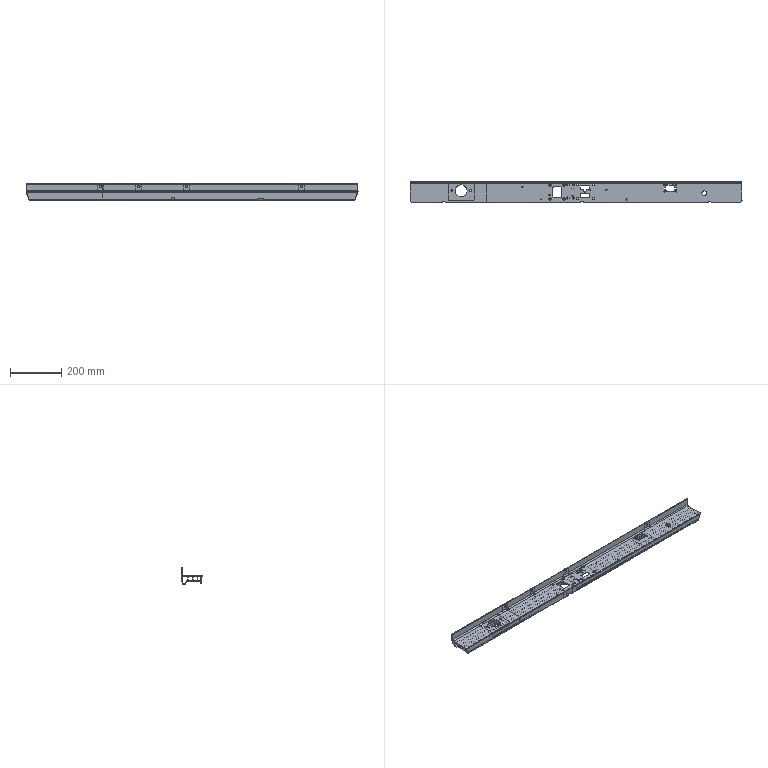NC program | NX | posted with a generic post | part box 1301 x 81.1 x 63 mm
Lines 1 to 1010 of 19512:
N10 G17 G21 G94 G90
(ZLEVEL_PROFILE , TOOL : D16)
N12 T16 M6
N14 G54
N16 G17 G0 G90 X661.143 Y51.891 B0. C0. S6000 M3
N18 G43 Z30. H16
N20 Z-0.968
N22 G94 G1 X659.105 Y50.713 F2000.
N24 G3 X658.305 Y49.328 R1.6
N26 G1 X658.306 Y41.58
N28 Y40.343
N30 X658.31 Y40.291
N32 Y32.645
N34 X658.306 Y32.615
N36 Y28.583
N38 X658.286 Y28.102
N40 G3 X659.029 Y26.685 R1.6
N42 G1 X661.071 Y25.392
N44 G0 Y25.391 Z-1.935
N46 G1 X659.029 Y26.685
N48 G2 X658.286 Y28.102 R1.6
N50 G1 X658.306 Y28.583
N52 Y32.615
N54 X658.31 Y32.645
N56 Y40.291
N58 X658.306 Y40.343
N60 Y41.58
N62 X658.305 Y49.328
N64 G2 X659.105 Y50.713 R1.6
N66 G1 X661.143 Y51.891
N68 G0 X661.144 Z-2.903
N70 G1 X659.105 Y50.713
N72 G3 X658.305 Y49.328 R1.6
N74 G1 X658.306 Y41.58
N76 X658.307 Y40.343
N78 X658.31 Y40.291
N80 Y32.645
N82 X658.306 Y32.615
N84 Y28.583
N86 X658.287 Y28.102
N88 G3 X659.029 Y26.684 R1.6
N90 G1 X661.071 Y25.391
N92 G0 Z-3.871
N94 G1 X659.029 Y26.684
N96 G2 X658.287 Y28.102 R1.6
N98 G1 X658.306 Y28.583
N100 X658.307 Y32.615
N102 X658.31 Y32.645
N104 Y40.291
N106 X658.307 Y40.343
N108 X658.306 Y41.58
N110 X658.305 Y49.328
N112 G2 X659.105 Y50.713 R1.6
N114 G1 X661.144 Y51.891
N116 G0 Z-4.839
N118 G1 X659.105 Y50.713
N120 G3 X658.305 Y49.328 R1.6
N122 G1 X658.306 Y41.58
N124 X658.307 Y40.343
N126 X658.31 Y40.291
N128 Y32.645
N130 X658.307 Y32.615
N132 Y28.583
N134 X658.287 Y28.102
N136 G3 X659.029 Y26.684 R1.6
N138 G1 X661.071 Y25.39
N140 G0 Z-5.806
N142 G1 X659.029 Y26.684
N144 G2 X658.287 Y28.102 R1.6
N146 G1 X658.307 Y28.583
N148 Y32.615
N150 X658.31 Y32.645
N152 Y40.291
N154 X658.307 Y40.343
N156 X658.306 Y41.58
N158 X658.305 Y49.328
N160 G2 X659.105 Y50.713 R1.6
N162 G1 X661.144 Y51.891
N164 G0 Z-6.774
N166 G1 X659.105 Y50.713
N168 G3 X658.305 Y49.328 R1.6
N170 G1 X658.306 Y41.58
N172 X658.307 Y40.343
N174 X658.31 Y40.291
N176 Y32.645
N178 X658.307 Y32.615
N180 Y28.583
N182 X658.287 Y28.102
N184 G3 X659.029 Y26.684 R1.6
N186 G1 X661.07 Y25.389
N188 G0 Z-7.742
N190 G1 X659.029 Y26.684
N192 G2 X658.287 Y28.102 R1.6
N194 G1 X658.307 Y28.583
N196 Y32.615
N198 X658.31 Y32.645
N200 Y40.291
N202 X658.307 Y40.343
N204 X658.306 Y41.58
N206 X658.305 Y49.328
N208 G2 X659.105 Y50.713 R1.6
N210 G1 X661.144 Y51.891
N212 G0 Z-8.71
N214 G1 X659.105 Y50.713
N216 G3 X658.305 Y49.328 R1.6
N218 G1 X658.306 Y41.58
N220 X658.307 Y40.343
N222 X658.31 Y40.291
N224 Y32.645
N226 X658.307 Y32.615
N228 Y28.583
N230 X658.287 Y28.102
N232 G3 X659.028 Y26.684 R1.6
N234 G1 X661.07 Y25.388
N236 G0 Z-9.677
N238 G1 X659.028 Y26.684
N240 G2 X658.287 Y28.102 R1.6
N242 G1 X658.307 Y28.583
N244 Y32.615
N246 X658.31 Y32.645
N248 Y40.291
N250 X658.306 Y41.58
N252 X658.305 Y49.328
N254 G2 X659.105 Y50.713 R1.6
N256 G1 X661.144 Y51.891
N258 G0 Z-10.645
N260 G1 X659.105 Y50.713
N262 G3 X658.306 Y49.328 R1.6
N264 G1 Y41.58
N266 X658.31 Y40.291
N268 Y32.645
N270 X658.307 Y32.615
N272 X658.308 Y28.583
N274 X658.287 Y28.102
N276 G3 X659.028 Y26.684 R1.6
N278 G1 X661.07 Y25.387
N280 G0 Z-11.613
N282 G1 X659.028 Y26.684
N284 G2 X658.287 Y28.102 R1.6
N286 G1 X658.308 Y28.583
N288 X658.307 Y32.615
N290 X658.31 Y32.645
N292 X658.307 Y40.343
N294 X658.306 Y41.58
N296 Y49.328
N298 G2 X659.105 Y50.713 R1.6
N300 G1 X661.144 Y51.891
N302 G0 Z-12.581
N304 G1 X659.105 Y50.713
N306 G3 X658.306 Y49.328 R1.6
N308 G1 X658.307 Y41.58
N310 X658.31 Y40.291
N312 X658.307 Y32.615
N314 X658.308 Y28.583
N316 X658.287 Y28.102
N318 G3 X659.028 Y26.683 R1.6
N320 G1 X661.07 Y25.386
N322 G0 Z-13.548
N324 G1 X659.028 Y26.683
N326 G2 X658.288 Y28.102 R1.6
N328 G1 X658.308 Y28.583
N330 X658.31 Y32.645
N332 X658.308 Y40.343
N334 X658.307 Y41.58
N336 X658.306 Y49.328
N338 G2 X659.106 Y50.713 R1.6
N340 G1 X661.144 Y51.891
N342 G0 X661.145 Z-14.516
N344 G1 X659.106 Y50.713
N346 G3 X658.306 Y49.328 R1.6
N348 G1 X658.307 Y41.58
N350 X658.31 Y40.291
N352 X658.308 Y32.615
N354 Y28.583
N356 X658.288 Y28.102
N358 G3 X659.028 Y26.683 R1.6
N360 G1 X661.07 Y25.385
N362 G0 Z-15.484
N364 G1 X659.028 Y26.683
N366 G2 X658.288 Y28.102 R1.6
N368 G1 X658.308 Y28.583
N370 X658.31 Y32.645
N372 X658.308 Y40.343
N374 X658.307 Y41.58
N376 X658.306 Y49.328
N378 G2 X659.106 Y50.713 R1.6
N380 G1 X661.145 Y51.891
N382 G0 Z-16.452
N384 G1 X659.106 Y50.713
N386 G3 X658.306 Y49.328 R1.6
N388 G1 X658.307 Y41.58
N390 X658.31 Y40.291
N392 X658.308 Y32.615
N394 X658.309 Y28.583
N396 X658.288 Y28.102
N398 G3 X659.028 Y26.683 R1.6
N400 G1 X661.07 Y25.384
N402 G0 Z-17.419
N404 G1 X659.028 Y26.683
N406 G2 X658.288 Y28.102 R1.6
N408 G1 X658.309 Y28.583
N410 X658.31 Y32.645
N412 X658.308 Y40.343
N414 X658.307 Y41.58
N416 X658.306 Y49.328
N418 G2 X659.106 Y50.713 R1.6
N420 G1 X661.145 Y51.891
N422 G0 Z-18.387
N424 G1 X659.106 Y50.713
N426 G3 X658.306 Y49.328 R1.6
N428 G1 X658.307 Y41.58
N430 X658.31 Y40.291
N432 X658.308 Y32.615
N434 X658.309 Y28.583
N436 X658.288 Y28.102
N438 G3 X659.027 Y26.683 R1.6
N440 G1 X661.07 Y25.383
N442 G0 X661.069 Z-19.355
N444 G1 X659.027 Y26.683
N446 G2 X658.288 Y28.102 R1.6
N448 G1 X658.309 Y28.583
N450 X658.31 Y32.645
N452 X658.308 Y40.343
N454 X658.307 Y41.58
N456 X658.306 Y49.328
N458 G2 X659.106 Y50.713 R1.6
N460 G1 X661.145 Y51.891
N462 G0 Z-20.323
N464 G1 X659.106 Y50.713
N466 G3 X658.306 Y49.328 R1.6
N468 G1 X658.307 Y41.58
N470 X658.31 Y40.291
N472 X658.308 Y32.615
N474 X658.309 Y28.583
N476 X658.288 Y28.102
N478 G3 X659.027 Y26.683 R1.6
N480 G1 X661.069 Y25.382
N482 G0 Z-21.29
N484 G1 X659.027 Y26.683
N486 G2 X658.288 Y28.102 R1.6
N488 G1 X658.309 Y28.583
N490 X658.31 Y32.645
N492 X658.308 Y40.343
N494 X658.307 Y41.58
N496 X658.306 Y49.328
N498 G2 X659.106 Y50.713 R1.6
N500 G1 X661.145 Y51.891
N502 G0 Z-22.258
N504 G1 X659.106 Y50.713
N506 G3 X658.306 Y49.328 R1.6
N508 G1 X658.307 Y41.58
N510 X658.31 Y40.291
N512 X658.308 Y32.615
N514 X658.309 Y28.583
N516 X658.288 Y28.102
N518 G3 X659.027 Y26.683 R1.6
N520 G1 X661.069 Y25.381
N522 G0 Z-23.226
N524 G1 X659.027 Y26.682
N526 G2 X658.288 Y28.102 R1.6
N528 G1 X658.31 Y28.583
N530 Y32.645
N532 Y40.291
N534 X658.307 Y41.58
N536 X658.306 Y49.328
N538 G2 X659.106 Y50.713 R1.6
N540 G1 X661.145 Y51.891
N542 G0 Z-24.194
N544 G1 X659.106 Y50.713
N546 G3 X658.306 Y49.328 R1.6
N548 G1 X658.307 Y41.58
N550 X658.31 Y40.291
N552 Y32.645
N554 Y28.583
N556 X658.289 Y28.102
N558 G3 X659.027 Y26.682 R1.6
N560 G1 X661.069 Y25.38
N562 G0 X661.07 Y25.383 Z-25.161
N564 G1 X659.028 Y26.683
N566 G2 X658.289 Y28.102 R1.6
N568 G1 X658.31 Y28.583
N570 Y32.645
N572 Y40.291
N574 X658.307 Y41.58
N576 Y49.328
N578 G2 X659.106 Y50.713 R1.6
N580 G1 X661.146 Y51.891
N582 G0 Z-26.129
N584 G1 X659.106 Y50.713
N586 G3 X658.307 Y49.328 R1.6
N588 G1 Y41.58
N590 X658.31 Y40.291
N592 Y32.645
N594 Y28.583
N596 X658.289 Y28.102
N598 G3 X659.03 Y26.683 R1.6
N600 G1 X661.072 Y25.386
N602 G0 X661.073 Y25.39 Z-27.097
N604 G1 X659.032 Y26.684
N606 G2 X658.29 Y28.102 R1.6
N608 G1 X658.31 Y28.583
N610 Y32.645
N612 Y40.291
N614 X658.307 Y41.58
N616 Y49.328
N618 G2 X659.107 Y50.713 R1.6
N620 G1 X661.146 Y51.89
N622 G0 Z-28.065
N624 G1 X659.107 Y50.713
N626 G3 X658.307 Y49.328 R1.6
N628 G1 Y41.58
N630 X658.31 Y40.291
N632 Y32.645
N634 Y28.583
N636 X658.29 Y28.102
N638 G3 X659.034 Y26.685 R1.6
N640 G1 X661.076 Y25.393
N642 G0 X661.079 Y25.395 Z-29.032
N644 G1 X659.035 Y26.686
N646 G2 X658.291 Y28.102 R1.6
N648 G1 X658.31 Y28.583
N650 Y32.645
N652 Y40.291
N654 X658.307 Y41.58
N656 X658.305 Y49.719
N658 G2 X659.105 Y51.105 R1.6
N660 G1 X661.146 Y52.284
N662 G0 X661.141 Y52.704 Z-30.
N664 G1 X659.104 Y51.527
N666 G3 X658.305 Y50.141 R1.6
N668 G1 X658.307 Y41.58
N670 X658.31 Y40.317
N672 Y32.402
N674 Y28.583
N676 X658.291 Y28.102
N678 G3 X659.037 Y26.686 R1.6
N680 G1 X661.082 Y25.398
N682 G0 Z30.
N684 X-661.062 Y25.372
N686 Z-0.968
N688 G1 X-659.019 Y26.681
N690 G3 X-658.284 Y28.102 R1.6
N692 G1 X-658.306 Y28.583
N694 Y33.818
N696 X-658.31 Y33.848
N698 Y40.291
N700 X-658.306 Y41.58
N702 X-658.305 Y49.328
N704 G3 X-659.105 Y50.713 R1.6
N706 G1 X-661.143 Y51.891
N708 G0 Z-1.935
N710 G1 X-659.105 Y50.713
N712 G2 X-658.305 Y49.328 R1.6
N714 G1 X-658.306 Y41.58
N716 X-658.31 Y40.291
N718 Y33.848
N720 X-658.306 Y33.818
N722 Y28.583
N724 X-658.284 Y28.102
N726 G2 X-659.019 Y26.681 R1.6
N728 G1 X-661.062 Y25.372
N730 G0 Z-2.903
N732 G1 X-659.02 Y26.681
N734 G3 X-658.284 Y28.102 R1.6
N736 G1 X-658.306 Y28.583
N738 Y33.818
N740 X-658.31 Y33.848
N742 Y40.291
N744 X-658.306 Y41.58
N746 X-658.305 Y49.328
N748 G3 X-659.105 Y50.713 R1.6
N750 G1 X-661.144 Y51.891
N752 G0 Z-3.871
N754 G1 X-659.105 Y50.713
N756 G2 X-658.305 Y49.328 R1.6
N758 G1 X-658.306 Y41.58
N760 X-658.31 Y40.291
N762 Y33.848
N764 X-658.307 Y33.818
N766 X-658.306 Y28.583
N768 X-658.284 Y28.102
N770 G2 X-659.02 Y26.681 R1.6
N772 G1 X-661.063 Y25.373
N774 G0 X-661.064 Y25.372 Z-4.839
N776 G1 X-659.02 Y26.681
N778 G3 X-658.285 Y28.102 R1.6
N780 G1 X-658.307 Y28.583
N782 Y33.818
N784 X-658.31 Y33.848
N786 Y40.291
N788 X-658.306 Y41.58
N790 X-658.305 Y49.328
N792 G3 X-659.105 Y50.713 R1.6
N794 G1 X-661.144 Y51.891
N796 G0 Z-5.806
N798 G1 X-659.105 Y50.713
N800 G2 X-658.305 Y49.328 R1.6
N802 G1 X-658.306 Y41.58
N804 X-658.31 Y40.291
N806 Y33.848
N808 X-658.307 Y33.818
N810 Y28.583
N812 X-658.285 Y28.102
N814 G2 X-659.02 Y26.681 R1.6
N816 G1 X-661.064 Y25.372
N818 G0 Y25.373 Z-6.774
N820 G1 X-659.02 Y26.681
N822 G3 X-658.285 Y28.102 R1.6
N824 G1 X-658.307 Y28.583
N826 Y33.818
N828 X-658.31 Y33.848
N830 Y40.291
N832 X-658.306 Y41.58
N834 X-658.305 Y49.328
N836 G3 X-659.105 Y50.713 R1.6
N838 G1 X-661.144 Y51.891
N840 G0 Z-7.742
N842 G1 X-659.105 Y50.713
N844 G2 X-658.305 Y49.328 R1.6
N846 G1 X-658.306 Y41.58
N848 X-658.31 Y40.291
N850 Y33.848
N852 X-658.307 Y33.818
N854 Y28.583
N856 X-658.285 Y28.102
N858 G2 X-659.021 Y26.681 R1.6
N860 G1 X-661.064 Y25.373
N862 G0 Z-8.71
N864 G1 X-659.021 Y26.681
N866 G3 X-658.285 Y28.102 R1.6
N868 G1 X-658.307 Y28.583
N870 Y33.818
N872 X-658.31 Y33.848
N874 Y40.291
N876 X-658.306 Y41.58
N878 X-658.305 Y49.328
N880 G3 X-659.105 Y50.713 R1.6
N882 G1 X-661.144 Y51.891
N884 G0 Z-9.677
N886 G1 X-659.105 Y50.713
N888 G2 X-658.306 Y49.328 R1.6
N890 G1 Y41.58
N892 X-658.31 Y40.291
N894 Y33.848
N896 X-658.307 Y33.818
N898 Y28.583
N900 X-658.285 Y28.102
N902 G2 X-659.021 Y26.681 R1.6
N904 G1 X-661.064 Y25.373
N906 G0 X-661.065 Y25.374 Z-10.645
N908 G1 X-659.021 Y26.681
N910 G3 X-658.286 Y28.102 R1.6
N912 G1 X-658.308 Y28.583
N914 X-658.307 Y33.818
N916 X-658.31 Y33.848
N918 Y40.291
N920 X-658.306 Y41.58
N922 Y49.328
N924 G3 X-659.105 Y50.713 R1.6
N926 G1 X-661.144 Y51.891
N928 G0 Z-11.613
N930 G1 X-659.105 Y50.713
N932 G2 X-658.306 Y49.328 R1.6
N934 G1 Y41.58
N936 X-658.31 Y40.291
N938 X-658.307 Y33.818
N940 X-658.308 Y28.583
N942 X-658.286 Y28.102
N944 G2 X-659.022 Y26.681 R1.6
N946 G1 X-661.065 Y25.374
N948 G0 Z-12.581
N950 G1 X-659.022 Y26.681
N952 G3 X-658.286 Y28.102 R1.6
N954 G1 X-658.308 Y28.583
N956 X-658.31 Y33.848
N958 Y40.291
N960 X-658.307 Y41.58
N962 X-658.306 Y49.328
N964 G3 X-659.106 Y50.713 R1.6
N966 G1 X-661.144 Y51.891
N968 G0 X-661.145 Z-13.548
N970 G1 X-659.106 Y50.713
N972 G2 X-658.306 Y49.328 R1.6
N974 G1 X-658.307 Y41.58
N976 X-658.31 Y40.291
N978 X-658.307 Y33.818
N980 X-658.308 Y28.583
N982 X-658.286 Y28.102
N984 G2 X-659.022 Y26.681 R1.6
N986 G1 X-661.065 Y25.374
N988 G0 Z-14.516
N990 G1 X-659.022 Y26.681
N992 G3 X-658.286 Y28.102 R1.6
N994 G1 X-658.308 Y28.583
N996 X-658.31 Y33.848
N998 Y40.291
N1000 X-658.307 Y41.58
N1002 X-658.306 Y49.328
N1004 G3 X-659.106 Y50.713 R1.6
N1006 G1 X-661.145 Y51.891
N1008 G0 Z-15.484
N1010 G1 X-659.106 Y50.713
N1012 G2 X-658.306 Y49.328 R1.6
N1014 G1 X-658.307 Y41.58
N1016 X-658.31 Y40.291
N1018 Y33.848
N1020 X-658.308 Y28.583
N1022 X-658.286 Y28.102
N1024 G2 X-659.023 Y26.681 R1.6
N1026 G1 X-661.066 Y25.375
N1028 G0 Z-16.452
N1030 G1 X-659.023 Y26.681
N1032 G3 X-658.287 Y28.102 R1.6
N1034 G1 X-658.309 Y28.583
N1036 X-658.31 Y33.848
N1038 Y40.291
N1040 X-658.307 Y41.58
N1042 X-658.306 Y49.328
N1044 G3 X-659.106 Y50.713 R1.6
N1046 G1 X-661.145 Y51.891
N1048 G0 Z-17.419
N1050 G1 X-659.106 Y50.713
N1052 G2 X-658.306 Y49.328 R1.6
N1054 G1 X-658.307 Y41.58
N1056 X-658.31 Y40.291
N1058 Y33.848
N1060 X-658.309 Y28.583
N1062 X-658.287 Y28.102
N1064 G2 X-659.023 Y26.681 R1.6
N1066 G1 X-661.066 Y25.375
N1068 G0 Z-18.387
N1070 G1 X-659.023 Y26.681
N1072 G3 X-658.287 Y28.102 R1.6
N1074 G1 X-658.309 Y28.583
N1076 X-658.31 Y33.848
N1078 Y40.291
N1080 X-658.307 Y41.58
N1082 X-658.306 Y49.328
N1084 G3 X-659.106 Y50.713 R1.6
N1086 G1 X-661.145 Y51.891
N1088 G0 Z-19.355
N1090 G1 X-659.106 Y50.713
N1092 G2 X-658.306 Y49.328 R1.6
N1094 G1 X-658.307 Y41.58
N1096 X-658.31 Y40.291
N1098 Y33.848
N1100 X-658.309 Y28.583
N1102 X-658.287 Y28.102
N1104 G2 X-659.024 Y26.681 R1.6
N1106 G1 X-661.066 Y25.375
N1108 G0 X-661.067 Y25.376 Z-20.323
N1110 G1 X-659.024 Y26.681
N1112 G3 X-658.287 Y28.102 R1.6
N1114 G1 X-658.309 Y28.583
N1116 X-658.31 Y33.848
N1118 Y40.291
N1120 X-658.307 Y41.58
N1122 X-658.306 Y49.328
N1124 G3 X-659.106 Y50.713 R1.6
N1126 G1 X-661.145 Y51.891
N1128 G0 Z-21.29
N1130 G1 X-659.106 Y50.713
N1132 G2 X-658.306 Y49.328 R1.6
N1134 G1 X-658.307 Y41.58
N1136 X-658.31 Y40.291
N1138 X-658.308 Y33.818
N1140 X-658.309 Y28.583
N1142 X-658.288 Y28.102
N1144 G2 X-659.024 Y26.681 R1.6
N1146 G1 X-661.067 Y25.376
N1148 G0 Z-22.258
N1150 G1 X-659.024 Y26.681
N1152 G3 X-658.288 Y28.102 R1.6
N1154 G1 X-658.309 Y28.583
N1156 X-658.31 Y33.848
N1158 Y40.291
N1160 X-658.307 Y41.58
N1162 X-658.306 Y49.328
N1164 G3 X-659.106 Y50.713 R1.6
N1166 G1 X-661.145 Y51.891
N1168 G0 Z-23.226
N1170 G1 X-659.106 Y50.713
N1172 G2 X-658.306 Y49.328 R1.6
N1174 G1 X-658.307 Y41.58
N1176 X-658.31 Y40.291
N1178 X-658.308 Y33.818
N1180 X-658.31 Y28.583
N1182 X-658.288 Y28.102
N1184 G2 X-659.025 Y26.682 R1.6
N1186 G1 X-661.067 Y25.376
N1188 G0 X-661.068 Z-24.194
N1190 G1 X-659.025 Y26.682
N1192 G3 X-658.288 Y28.102 R1.6
N1194 G1 X-658.31 Y28.583
N1196 Y33.848
N1198 Y40.291
N1200 X-658.307 Y41.58
N1202 X-658.306 Y49.328
N1204 G3 X-659.106 Y50.713 R1.6
N1206 G1 X-661.145 Y51.891
N1208 G0 X-661.146 Z-25.161
N1210 G1 X-659.106 Y50.713
N1212 G2 X-658.307 Y49.328 R1.6
N1214 G1 Y41.58
N1216 X-658.31 Y40.291
N1218 X-658.309 Y33.818
N1220 X-658.31 Y28.583
N1222 X-658.288 Y28.102
N1224 G2 X-659.025 Y26.682 R1.6
N1226 G1 X-661.068 Y25.377
N1228 G0 Z-26.129
N1230 G1 X-659.025 Y26.682
N1232 G3 X-658.288 Y28.102 R1.6
N1234 G1 X-658.31 Y28.583
N1236 Y33.848
N1238 Y40.291
N1240 X-658.307 Y41.58
N1242 Y49.328
N1244 G3 X-659.107 Y50.713 R1.6
N1246 G1 X-661.146 Y51.891
N1248 G0 Z-27.097
N1250 G1 X-659.107 Y50.713
N1252 G2 X-658.307 Y49.328 R1.6
N1254 G1 Y41.58
N1256 X-658.31 Y40.291
N1258 X-658.309 Y33.818
N1260 X-658.31 Y28.583
N1262 X-658.288 Y28.102
N1264 G2 X-659.026 Y26.682 R1.6
N1266 G1 X-661.068 Y25.378
N1268 G0 X-661.07 Y25.377 Z-28.065
N1270 G1 X-659.026 Y26.682
N1272 G3 X-658.288 Y28.102 R1.6
N1274 G1 X-658.31 Y28.583
N1276 Y33.848
N1278 Y40.291
N1280 X-658.307 Y41.58
N1282 Y49.328
N1284 G3 X-659.107 Y50.713 R1.6
N1286 G1 X-661.146 Y51.891
N1288 G0 X-661.147 Y52.284 Z-29.032
N1290 G1 X-659.105 Y51.105
N1292 G2 X-658.305 Y49.719 R1.6
N1294 G1 X-658.307 Y41.58
N1296 X-658.31 Y40.291
N1298 X-658.309 Y33.818
N1300 X-658.31 Y28.583
N1302 X-658.288 Y28.102
N1304 G2 X-659.026 Y26.682 R1.6
N1306 G1 X-661.069 Y25.379
N1308 G0 X-661.07 Z-30.
N1310 G1 X-659.027 Y26.682
N1312 G3 X-658.289 Y28.102 R1.6
N1314 G1 X-658.31 Y28.583
N1316 Y32.402
N1318 Y40.317
N1320 X-658.307 Y41.58
N1322 X-658.305 Y50.141
N1324 G3 X-659.104 Y51.527 R1.6
N1326 G1 X-661.141 Y52.703
N1328 G0 Z30.
(ZLEVEL_PROFILE_COPY , TOOL : D16)
N1330 X661.311 Y51.495
N1332 Z-31.
N1334 G1 X659.106 Y50.221
N1336 G3 X658.306 Y48.835 R1.6
N1338 G1 X658.307 Y41.022
N1340 X658.31 Y40.55
N1342 Y-40.472
N1344 X658.306 Y-40.503
N1346 X658.308 Y-48.835
N1348 G3 X659.108 Y-50.221 R1.6
N1350 G1 X661.313 Y-51.493
N1352 G0 X661.314 Z-32.
N1354 G1 X659.109 Y-50.221
N1356 G2 X658.308 Y-48.835 R1.6
N1358 G1 X658.306 Y-40.503
N1360 X658.31 Y-40.472
N1362 Y40.55
N1364 X658.307 Y41.022
N1366 X658.306 Y48.835
N1368 G2 X659.106 Y50.221 R1.6
N1370 G1 X661.311 Y51.494
N1372 G0 Z-33.
N1374 G1 X659.106 Y50.221
N1376 G3 X658.306 Y48.835 R1.6
N1378 G1 X658.307 Y41.022
N1380 X658.31 Y40.55
N1382 Y-40.472
N1384 X658.307 Y-40.503
N1386 X658.309 Y-48.835
N1388 G3 X659.109 Y-50.221 R1.6
N1390 G1 X661.314 Y-51.493
N1392 G0 Z30.
N1394 X-661.313
N1396 Z-31.
N1398 G1 X-659.108 Y-50.221
N1400 G3 X-658.308 Y-48.835 R1.6
N1402 G1 X-658.306 Y-40.442
N1404 X-658.31 Y-40.411
N1406 Y40.55
N1408 X-658.307 Y41.022
N1410 X-658.306 Y48.835
N1412 G3 X-659.106 Y50.221 R1.6
N1414 G1 X-661.311 Y51.495
N1416 G0 Y51.494 Z-32.
N1418 G1 X-659.106 Y50.221
N1420 G2 X-658.306 Y48.835 R1.6
N1422 G1 X-658.307 Y41.022
N1424 X-658.31 Y40.55
N1426 Y-40.411
N1428 X-658.306 Y-40.442
N1430 X-658.308 Y-48.835
N1432 G2 X-659.109 Y-50.221 R1.6
N1434 G1 X-661.314 Y-51.493
N1436 G0 Z-33.
N1438 G1 X-659.109 Y-50.221
N1440 G3 X-658.309 Y-48.835 R1.6
N1442 G1 X-658.307 Y-40.442
N1444 X-658.31 Y-40.411
N1446 Y40.55
N1448 X-658.307 Y41.022
N1450 X-658.306 Y48.835
N1452 G3 X-659.106 Y50.221 R1.6
N1454 G1 X-661.311 Y51.494
N1456 G0 Z30.
(CAVITY_MILL , TOOL : D16)
N1458 X-508.199 Y51.45 S9500
N1460 Z0.503
N1462 G1 Z-0.997 F1000.
N1464 X-513.915 Y41.55
N1466 G2 X-514.781 Y41.05 R1.
N1468 G1 X-650.31 F2500.
N1470 G3 X-651.11 Y40.263 R0.8
N1472 G1 Y37.25
N1474 G3 X-650.555 Y36.488 R0.8
N1476 G1 X-650.36 Y36.452
N1478 X-650.256 Y36.45
N1480 X-379.249
N1482 G3 X-375.264 Y29.25 R10.073
N1484 G1 X-370.486
N1486 G2 X-377.365 Y37.25 R8.153
N1488 G1 Y40.25
N1490 G2 X-370.519 Y48.25 R8.116
N1492 G1 X-375.288
N1494 G3 X-379.252 Y41.05 R10.036
N1496 G1 X-514.781
N1498 G2 X-515.647 Y41.55 R1.
N1500 G1 X-521.363 Y51.45
N1502 Z0.503
N1504 G0 X-508.483 Z-0.493
N1506 G1 Z-1.993 F1000.
N1508 X-514.199 Y41.55
N1510 G2 X-515.065 Y41.05 R1.
N1512 G1 X-650.31 F2500.
N1514 G3 X-651.11 Y40.263 R0.8
N1516 G1 Y37.25
N1518 G3 X-650.555 Y36.488 R0.8
N1520 G1 X-650.36 Y36.452
N1522 X-650.256 Y36.45
N1524 X-379.818
N1526 G3 X-375.855 Y29.25 R10.041
N1528 G1 X-371.1
N1530 G2 X-377.931 Y37.25 R8.121
N1532 G1 Y40.25
N1534 G2 X-371.097 Y48.25 R8.103
N1536 G1 X-375.863
N1538 G3 X-379.819 Y41.05 R10.023
N1540 G1 X-515.065
N1542 G2 X-515.931 Y41.55 R1.
N1544 G1 X-521.647 Y51.45
N1546 Z-0.493
N1548 G0 X-508.567 Z-1.49
N1550 G1 Z-2.99 F1000.
N1552 X-514.283 Y41.55
N1554 G2 X-515.149 Y41.05 R1.
N1556 G1 X-650.31 F2500.
N1558 G3 X-651.11 Y40.263 R0.8
N1560 G1 Y37.25
N1562 G3 X-650.555 Y36.488 R0.8
N1564 G1 X-650.36 Y36.452
N1566 X-650.256 Y36.45
N1568 X-379.987
N1570 G3 X-376.032 Y29.25 R10.021
N1572 G1 X-371.267
N1574 G2 X-378.098 Y37.162 R8.101
N1576 G1 X-378.099 Y40.278
N1578 G2 X-371.267 Y48.25 R8.101
N1580 G1 X-376.032
N1582 G3 X-379.987 Y41.05 R10.021
N1584 G1 X-515.149
N1586 G2 X-516.015 Y41.55 R1.
N1588 G1 X-521.731 Y51.45
N1590 Z-1.49
N1592 G0 X-508.567 Z-2.487
N1594 G1 Z-3.987 F1000.
N1596 X-514.283 Y41.55
N1598 G2 X-515.149 Y41.05 R1.
N1600 G1 X-650.31 F2500.
N1602 G3 X-651.11 Y40.263 R0.8
N1604 G1 Y37.25
N1606 G3 X-650.555 Y36.488 R0.8
N1608 G1 X-650.36 Y36.452
N1610 X-650.256 Y36.45
N1612 X-379.987
N1614 G3 X-376.033 Y29.25 R10.02
N1616 G1 X-371.268
N1618 G2 X-378.099 Y37.25 R8.1
N1620 G1 Y40.25
N1622 G2 X-371.268 Y48.25 R8.1
N1624 G1 X-376.033
N1626 G3 X-379.987 Y41.05 R10.02
N1628 G1 X-515.149
N1630 G2 X-516.015 Y41.55 R1.
N1632 G1 X-521.731 Y51.45
N1634 Z-2.487
N1636 G0 X-508.567 Z-3.483
N1638 G1 Z-4.983 F1000.
N1640 X-514.283 Y41.55
N1642 G2 X-515.149 Y41.05 R1.
N1644 G1 X-650.31 F2500.
N1646 G3 X-651.11 Y40.263 R0.8
N1648 G1 Y37.25
N1650 G3 X-650.555 Y36.488 R0.8
N1652 G1 X-650.36 Y36.452
N1654 X-650.256 Y36.45
N1656 X-379.987
N1658 G3 X-376.033 Y29.25 R10.02
N1660 G1 X-371.268
N1662 G2 X-378.099 Y37.25 R8.1
N1664 G1 Y40.25
N1666 G2 X-371.268 Y48.25 R8.1
N1668 G1 X-376.033
N1670 G3 X-379.987 Y41.05 R10.02
N1672 G1 X-515.149
N1674 G2 X-516.015 Y41.55 R1.
N1676 G1 X-521.731 Y51.45
N1678 Z-3.483
N1680 G0 X-508.567 Z-4.48
N1682 G1 Z-5.98 F1000.
N1684 X-514.283 Y41.55
N1686 G2 X-515.149 Y41.05 R1.
N1688 G1 X-650.31 F2500.
N1690 G3 X-651.11 Y40.263 R0.8
N1692 G1 Y37.25
N1694 G3 X-650.555 Y36.488 R0.8
N1696 G1 X-650.36 Y36.452
N1698 X-650.256 Y36.45
N1700 X-379.987
N1702 G3 X-376.033 Y29.25 R10.02
N1704 G1 X-371.268
N1706 G2 X-378.099 Y37.25 R8.1
N1708 G1 Y40.25
N1710 G2 X-371.268 Y48.25 R8.1
N1712 G1 X-376.033
N1714 G3 X-379.987 Y41.05 R10.02
N1716 G1 X-515.149
N1718 G2 X-516.015 Y41.55 R1.
N1720 G1 X-521.731 Y51.45
N1722 Z-4.48
N1724 G0 X-508.567 Z-5.477
N1726 G1 Z-6.977 F1000.
N1728 X-514.283 Y41.55
N1730 G2 X-515.149 Y41.05 R1.
N1732 G1 X-650.31 F2500.
N1734 G3 X-651.11 Y40.263 R0.8
N1736 G1 Y37.25
N1738 G3 X-650.555 Y36.488 R0.8
N1740 G1 X-650.36 Y36.452
N1742 X-650.256 Y36.45
N1744 X-379.987
N1746 G3 X-376.033 Y29.25 R10.02
N1748 G1 X-371.268
N1750 G2 X-378.099 Y37.25 R8.1
N1752 G1 Y40.25
N1754 G2 X-371.268 Y48.25 R8.1
N1756 G1 X-376.033
N1758 G3 X-379.987 Y41.05 R10.02
N1760 G1 X-515.149
N1762 G2 X-516.015 Y41.55 R1.
N1764 G1 X-521.731 Y51.45
N1766 Z-5.477
N1768 G0 X-508.567 Z-6.473
N1770 G1 Z-7.973 F1000.
N1772 X-514.283 Y41.55
N1774 G2 X-515.149 Y41.05 R1.
N1776 G1 X-650.31 F2500.
N1778 G3 X-651.11 Y40.263 R0.8
N1780 G1 Y37.25
N1782 G3 X-650.555 Y36.488 R0.8
N1784 X-650.358 Y36.451 R0.8
N1786 G1 X-650.258 Y36.45
N1788 X-379.987
N1790 G3 X-376.033 Y29.25 R10.02
N1792 G1 X-371.268
N1794 G2 X-378.099 Y37.25 R8.1
N1796 G1 Y40.25
N1798 G2 X-371.268 Y48.25 R8.1
N1800 G1 X-376.033
N1802 G3 X-379.987 Y41.05 R10.02
N1804 G1 X-515.149
N1806 G2 X-516.015 Y41.55 R1.
N1808 G1 X-521.731 Y51.45
N1810 Z-6.473
N1812 G0 X-508.567 Z-7.47
N1814 G1 Z-8.97 F1000.
N1816 X-514.283 Y41.55
N1818 G2 X-515.149 Y41.05 R1.
N1820 G1 X-650.31 F2500.
N1822 G3 X-651.11 Y40.263 R0.8
N1824 G1 Y37.25
N1826 G3 X-650.555 Y36.488 R0.8
N1828 X-650.358 Y36.451 R0.8
N1830 G1 X-650.258 Y36.45
N1832 X-379.987
N1834 G3 X-376.033 Y29.25 R10.02
N1836 G1 X-371.268
N1838 G2 X-378.099 Y37.25 R8.1
N1840 G1 Y40.25
N1842 G2 X-371.268 Y48.25 R8.1
N1844 G1 X-376.033
N1846 G3 X-379.987 Y41.05 R10.02
N1848 G1 X-515.149
N1850 G2 X-516.015 Y41.55 R1.
N1852 G1 X-521.731 Y51.45
N1854 Z-7.47
N1856 G0 X-508.567 Z-8.467
N1858 G1 Z-9.967 F1000.
N1860 X-514.283 Y41.55
N1862 G2 X-515.149 Y41.05 R1.
N1864 G1 X-650.31 F2500.
N1866 G3 X-651.11 Y40.263 R0.8
N1868 G1 Y37.25
N1870 G3 X-650.555 Y36.488 R0.8
N1872 X-650.358 Y36.451 R0.8
N1874 G1 X-650.258 Y36.45
N1876 X-379.987
N1878 G3 X-376.033 Y29.25 R10.02
N1880 G1 X-371.268
N1882 G2 X-378.099 Y37.25 R8.1
N1884 G1 Y40.25
N1886 G2 X-371.268 Y48.25 R8.1
N1888 G1 X-376.033
N1890 G3 X-379.987 Y41.05 R10.02
N1892 G1 X-515.149
N1894 G2 X-516.015 Y41.55 R1.
N1896 G1 X-521.731 Y51.45
N1898 Z-8.467
N1900 G0 X-508.567 Z-9.463
N1902 G1 Z-10.963 F1000.
N1904 X-514.283 Y41.55
N1906 G2 X-515.149 Y41.05 R1.
N1908 G1 X-650.31 F2500.
N1910 G3 X-651.11 Y40.263 R0.8
N1912 G1 Y37.25
N1914 G3 X-650.555 Y36.488 R0.8
N1916 X-650.358 Y36.451 R0.8
N1918 G1 X-650.258 Y36.45
N1920 X-379.987
N1922 G3 X-376.033 Y29.25 R10.02
N1924 G1 X-371.268
N1926 G2 X-378.099 Y37.25 R8.1
N1928 G1 Y40.25
N1930 G2 X-371.268 Y48.25 R8.1
N1932 G1 X-376.033
N1934 G3 X-379.987 Y41.05 R10.02
N1936 G1 X-515.149
N1938 G2 X-516.015 Y41.55 R1.
N1940 G1 X-521.731 Y51.45
N1942 Z-9.463
N1944 G0 X-508.567 Z-10.46
N1946 G1 Z-11.96 F1000.
N1948 X-514.283 Y41.55
N1950 G2 X-515.149 Y41.05 R1.
N1952 G1 X-650.31 F2500.
N1954 G3 X-651.11 Y40.263 R0.8
N1956 G1 Y37.25
N1958 G3 X-650.555 Y36.488 R0.8
N1960 X-650.358 Y36.451 R0.8
N1962 G1 X-650.258 Y36.45
N1964 X-379.987
N1966 G3 X-376.033 Y29.25 R10.02
N1968 G1 X-371.268
N1970 G2 X-378.099 Y37.25 R8.1
N1972 G1 Y40.25
N1974 G2 X-371.268 Y48.25 R8.1
N1976 G1 X-376.033
N1978 G3 X-379.987 Y41.05 R10.02
N1980 G1 X-515.149
N1982 G2 X-516.015 Y41.55 R1.
N1984 G1 X-521.731 Y51.45
N1986 Z-10.46
N1988 G0 X-508.567 Z-11.457
N1990 G1 Z-12.957 F1000.
N1992 X-514.283 Y41.55
N1994 G2 X-515.149 Y41.05 R1.
N1996 G1 X-650.31 F2500.
N1998 G3 X-651.11 Y40.263 R0.8
N2000 G1 Y37.25
N2002 G3 X-650.555 Y36.488 R0.8
N2004 X-650.358 Y36.451 R0.8
N2006 G1 X-650.258 Y36.45